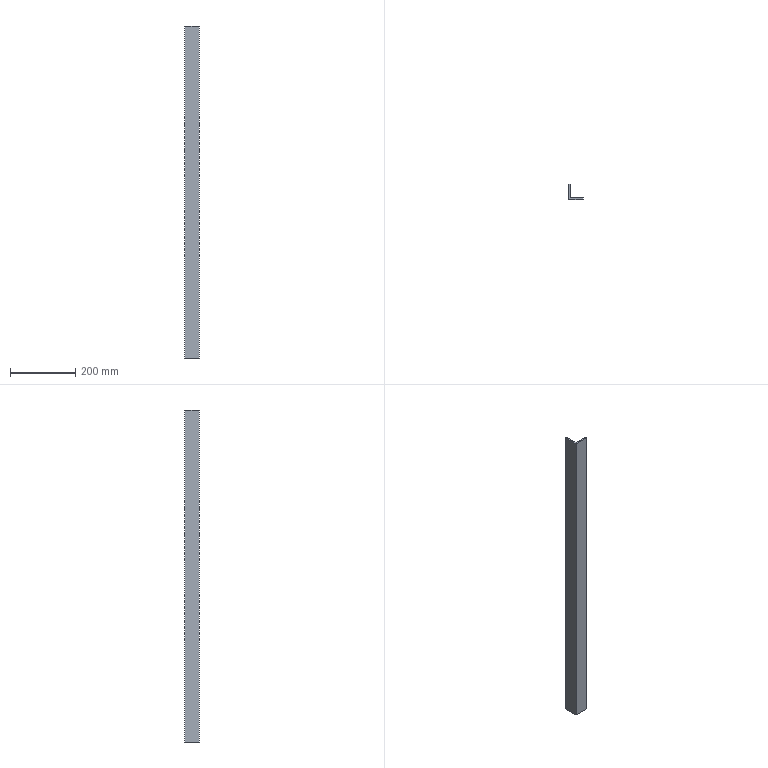Part | SolidWorks | features Extrusion 1 | 1 solid | 8 faces | box 45 x 45 x 1019 mm | volume 432947 mm3 | plane 8
STEP:
#1=CARTESIAN_POINT('',(-41.707,40.,0.));
#2=VERTEX_POINT('',#1);
#3=CARTESIAN_POINT('',(-46.707,40.,0.));
#4=VERTEX_POINT('',#3);
#5=CARTESIAN_POINT('',(-41.707,40.,0.));
#6=DIRECTION('',(-1.,0.,0.));
#7=VECTOR('',#6,1000.);
#8=LINE('',#5,#7);
#9=EDGE_CURVE('',#2,#4,#8,.T.);
#10=ORIENTED_EDGE('',*,*,#9,.T.);
#11=CARTESIAN_POINT('',(-46.707,40.,1018.7));
#12=VERTEX_POINT('',#11);
#13=CARTESIAN_POINT('',(-46.707,40.,1018.7));
#14=DIRECTION('',(0.,0.,-1.));
#15=VECTOR('',#14,1000.);
#16=LINE('',#13,#15);
#17=EDGE_CURVE('',#12,#4,#16,.T.);
#18=ORIENTED_EDGE('',*,*,#17,.F.);
#19=CARTESIAN_POINT('',(-41.707,40.,1018.7));
#20=VERTEX_POINT('',#19);
#21=CARTESIAN_POINT('',(-41.707,40.,1018.7));
#22=DIRECTION('',(-1.,0.,0.));
#23=VECTOR('',#22,1000.);
#24=LINE('',#21,#23);
#25=EDGE_CURVE('',#20,#12,#24,.T.);
#26=ORIENTED_EDGE('',*,*,#25,.F.);
#27=CARTESIAN_POINT('',(-41.707,40.,1018.7));
#28=DIRECTION('',(0.,0.,-1.));
#29=VECTOR('',#28,1000.);
#30=LINE('',#27,#29);
#31=EDGE_CURVE('',#20,#2,#30,.T.);
#32=ORIENTED_EDGE('',*,*,#31,.T.);
#33=EDGE_LOOP('',(#10,#18,#26,#32));
#34=FACE_OUTER_BOUND('',#33,.T.);
#35=CARTESIAN_POINT('',(-41.707,40.,1018.7));
#36=DIRECTION('',(0.,-1.,0.));
#37=DIRECTION('',(1.,0.,0.));
#38=AXIS2_PLACEMENT_3D('',#35,#36,#37);
#39=PLANE('',#38);
#40=ADVANCED_FACE('',(#34),#39,.F.);
#41=CARTESIAN_POINT('',(-46.707,-5.,0.));
#42=VERTEX_POINT('',#41);
#43=CARTESIAN_POINT('',(-46.707,40.,0.));
#44=DIRECTION('',(0.,-1.,0.));
#45=VECTOR('',#44,1000.);
#46=LINE('',#43,#45);
#47=EDGE_CURVE('',#4,#42,#46,.T.);
#48=ORIENTED_EDGE('',*,*,#47,.T.);
#49=CARTESIAN_POINT('',(-46.707,-5.,1018.7));
#50=VERTEX_POINT('',#49);
#51=CARTESIAN_POINT('',(-46.707,-5.,1018.7));
#52=DIRECTION('',(0.,0.,-1.));
#53=VECTOR('',#52,1000.);
#54=LINE('',#51,#53);
#55=EDGE_CURVE('',#50,#42,#54,.T.);
#56=ORIENTED_EDGE('',*,*,#55,.F.);
#57=CARTESIAN_POINT('',(-46.707,40.,1018.7));
#58=DIRECTION('',(0.,-1.,0.));
#59=VECTOR('',#58,1000.);
#60=LINE('',#57,#59);
#61=EDGE_CURVE('',#12,#50,#60,.T.);
#62=ORIENTED_EDGE('',*,*,#61,.F.);
#63=ORIENTED_EDGE('',*,*,#17,.T.);
#64=EDGE_LOOP('',(#48,#56,#62,#63));
#65=FACE_OUTER_BOUND('',#64,.T.);
#66=CARTESIAN_POINT('',(-46.707,40.,1018.7));
#67=DIRECTION('',(1.,0.,0.));
#68=DIRECTION('',(0.,1.,0.));
#69=AXIS2_PLACEMENT_3D('',#66,#67,#68);
#70=PLANE('',#69);
#71=ADVANCED_FACE('',(#65),#70,.F.);
#72=CARTESIAN_POINT('',(-1.707,-5.,0.));
#73=VERTEX_POINT('',#72);
#74=CARTESIAN_POINT('',(-46.707,-5.,0.));
#75=DIRECTION('',(1.,0.,0.));
#76=VECTOR('',#75,1000.);
#77=LINE('',#74,#76);
#78=EDGE_CURVE('',#42,#73,#77,.T.);
#79=ORIENTED_EDGE('',*,*,#78,.T.);
#80=CARTESIAN_POINT('',(-1.707,-5.,1018.7));
#81=VERTEX_POINT('',#80);
#82=CARTESIAN_POINT('',(-1.707,-5.,1018.7));
#83=DIRECTION('',(0.,0.,-1.));
#84=VECTOR('',#83,1000.);
#85=LINE('',#82,#84);
#86=EDGE_CURVE('',#81,#73,#85,.T.);
#87=ORIENTED_EDGE('',*,*,#86,.F.);
#88=CARTESIAN_POINT('',(-46.707,-5.,1018.7));
#89=DIRECTION('',(1.,0.,0.));
#90=VECTOR('',#89,1000.);
#91=LINE('',#88,#90);
#92=EDGE_CURVE('',#50,#81,#91,.T.);
#93=ORIENTED_EDGE('',*,*,#92,.F.);
#94=ORIENTED_EDGE('',*,*,#55,.T.);
#95=EDGE_LOOP('',(#79,#87,#93,#94));
#96=FACE_OUTER_BOUND('',#95,.T.);
#97=CARTESIAN_POINT('',(-46.707,-5.,1018.7));
#98=DIRECTION('',(0.,1.,0.));
#99=DIRECTION('',(0.,0.,1.));
#100=AXIS2_PLACEMENT_3D('',#97,#98,#99);
#101=PLANE('',#100);
#102=ADVANCED_FACE('',(#96),#101,.F.);
#103=CARTESIAN_POINT('',(-1.707,0.,0.));
#104=VERTEX_POINT('',#103);
#105=CARTESIAN_POINT('',(-1.707,-5.,0.));
#106=DIRECTION('',(0.,1.,0.));
#107=VECTOR('',#106,1000.);
#108=LINE('',#105,#107);
#109=EDGE_CURVE('',#73,#104,#108,.T.);
#110=ORIENTED_EDGE('',*,*,#109,.T.);
#111=CARTESIAN_POINT('',(-1.707,0.,1018.7));
#112=VERTEX_POINT('',#111);
#113=CARTESIAN_POINT('',(-1.707,0.,1018.7));
#114=DIRECTION('',(0.,0.,-1.));
#115=VECTOR('',#114,1000.);
#116=LINE('',#113,#115);
#117=EDGE_CURVE('',#112,#104,#116,.T.);
#118=ORIENTED_EDGE('',*,*,#117,.F.);
#119=CARTESIAN_POINT('',(-1.707,-5.,1018.7));
#120=DIRECTION('',(0.,1.,0.));
#121=VECTOR('',#120,1000.);
#122=LINE('',#119,#121);
#123=EDGE_CURVE('',#81,#112,#122,.T.);
#124=ORIENTED_EDGE('',*,*,#123,.F.);
#125=ORIENTED_EDGE('',*,*,#86,.T.);
#126=EDGE_LOOP('',(#110,#118,#124,#125));
#127=FACE_OUTER_BOUND('',#126,.T.);
#128=CARTESIAN_POINT('',(-1.707,-5.,1018.7));
#129=DIRECTION('',(-1.,0.,0.));
#130=DIRECTION('',(0.,0.,1.));
#131=AXIS2_PLACEMENT_3D('',#128,#129,#130);
#132=PLANE('',#131);
#133=ADVANCED_FACE('',(#127),#132,.F.);
#134=CARTESIAN_POINT('',(-41.707,0.,0.));
#135=VERTEX_POINT('',#134);
#136=CARTESIAN_POINT('',(-1.707,0.,0.));
#137=DIRECTION('',(-1.,0.,0.));
#138=VECTOR('',#137,1000.);
#139=LINE('',#136,#138);
#140=EDGE_CURVE('',#104,#135,#139,.T.);
#141=ORIENTED_EDGE('',*,*,#140,.T.);
#142=CARTESIAN_POINT('',(-41.707,0.,1018.7));
#143=VERTEX_POINT('',#142);
#144=CARTESIAN_POINT('',(-41.707,0.,1018.7));
#145=DIRECTION('',(0.,0.,-1.));
#146=VECTOR('',#145,1000.);
#147=LINE('',#144,#146);
#148=EDGE_CURVE('',#143,#135,#147,.T.);
#149=ORIENTED_EDGE('',*,*,#148,.F.);
#150=CARTESIAN_POINT('',(-1.707,0.,1018.7));
#151=DIRECTION('',(-1.,0.,0.));
#152=VECTOR('',#151,1000.);
#153=LINE('',#150,#152);
#154=EDGE_CURVE('',#112,#143,#153,.T.);
#155=ORIENTED_EDGE('',*,*,#154,.F.);
#156=ORIENTED_EDGE('',*,*,#117,.T.);
#157=EDGE_LOOP('',(#141,#149,#155,#156));
#158=FACE_OUTER_BOUND('',#157,.T.);
#159=CARTESIAN_POINT('',(-1.707,0.,1018.7));
#160=DIRECTION('',(0.,-1.,0.));
#161=DIRECTION('',(1.,0.,0.));
#162=AXIS2_PLACEMENT_3D('',#159,#160,#161);
#163=PLANE('',#162);
#164=ADVANCED_FACE('',(#158),#163,.F.);
#165=CARTESIAN_POINT('',(-41.707,0.,0.));
#166=DIRECTION('',(0.,1.,0.));
#167=VECTOR('',#166,1000.);
#168=LINE('',#165,#167);
#169=EDGE_CURVE('',#135,#2,#168,.T.);
#170=ORIENTED_EDGE('',*,*,#169,.T.);
#171=ORIENTED_EDGE('',*,*,#31,.F.);
#172=CARTESIAN_POINT('',(-41.707,0.,1018.7));
#173=DIRECTION('',(0.,1.,0.));
#174=VECTOR('',#173,1000.);
#175=LINE('',#172,#174);
#176=EDGE_CURVE('',#143,#20,#175,.T.);
#177=ORIENTED_EDGE('',*,*,#176,.F.);
#178=ORIENTED_EDGE('',*,*,#148,.T.);
#179=EDGE_LOOP('',(#170,#171,#177,#178));
#180=FACE_OUTER_BOUND('',#179,.T.);
#181=CARTESIAN_POINT('',(-41.707,0.,1018.7));
#182=DIRECTION('',(-1.,0.,0.));
#183=DIRECTION('',(0.,-1.,0.));
#184=AXIS2_PLACEMENT_3D('',#181,#182,#183);
#185=PLANE('',#184);
#186=ADVANCED_FACE('',(#180),#185,.F.);
#187=ORIENTED_EDGE('',*,*,#25,.T.);
#188=ORIENTED_EDGE('',*,*,#61,.T.);
#189=ORIENTED_EDGE('',*,*,#92,.T.);
#190=ORIENTED_EDGE('',*,*,#123,.T.);
#191=ORIENTED_EDGE('',*,*,#154,.T.);
#192=ORIENTED_EDGE('',*,*,#176,.T.);
#193=EDGE_LOOP('',(#187,#188,#189,#190,#191,#192));
#194=FACE_OUTER_BOUND('',#193,.T.);
#195=CARTESIAN_POINT('',(-46.707,40.,1018.7));
#196=DIRECTION('',(0.,0.,1.));
#197=DIRECTION('',(1.,0.,0.));
#198=AXIS2_PLACEMENT_3D('',#195,#196,#197);
#199=PLANE('',#198);
#200=ADVANCED_FACE('',(#194),#199,.T.);
#201=ORIENTED_EDGE('',*,*,#9,.F.);
#202=ORIENTED_EDGE('',*,*,#169,.F.);
#203=ORIENTED_EDGE('',*,*,#140,.F.);
#204=ORIENTED_EDGE('',*,*,#109,.F.);
#205=ORIENTED_EDGE('',*,*,#78,.F.);
#206=ORIENTED_EDGE('',*,*,#47,.F.);
#207=EDGE_LOOP('',(#201,#202,#203,#204,#205,#206));
#208=FACE_OUTER_BOUND('',#207,.T.);
#209=CARTESIAN_POINT('',(-46.707,40.,0.));
#210=DIRECTION('',(0.,0.,1.));
#211=DIRECTION('',(1.,0.,0.));
#212=AXIS2_PLACEMENT_3D('',#209,#210,#211);
#213=PLANE('',#212);
#214=ADVANCED_FACE('',(#208),#213,.F.);
#215=CLOSED_SHELL('',(#40,#71,#102,#133,#164,#186,#200,#214));
#216=MANIFOLD_SOLID_BREP('',#215);
#217=CARTESIAN_POINT('',(0.,0.,0.));
#218=DIRECTION('',(0.,0.,1.));
#219=DIRECTION('',(1.,0.,0.));
#220=AXIS2_PLACEMENT_3D('',#217,#218,#219);
#221=(LENGTH_UNIT()NAMED_UNIT(*)SI_UNIT(.MILLI.,.METRE.));
#222=UNCERTAINTY_MEASURE_WITH_UNIT(LENGTH_MEASURE(0.00001),#221,'','');
#223=(NAMED_UNIT(*)PLANE_ANGLE_UNIT()SI_UNIT($,.RADIAN.));
#224=(NAMED_UNIT(*)SI_UNIT($,.STERADIAN.)SOLID_ANGLE_UNIT());
#225=(GEOMETRIC_REPRESENTATION_CONTEXT(3)GLOBAL_UNCERTAINTY_ASSIGNED_CONTEXT((#222))GLOBAL_UNIT_ASSIGNED_CONTEXT((#221,#223,#224))REPRESENTATION_CONTEXT('',''));
#226=ADVANCED_BREP_SHAPE_REPRESENTATION('',(#216,#220),#225);